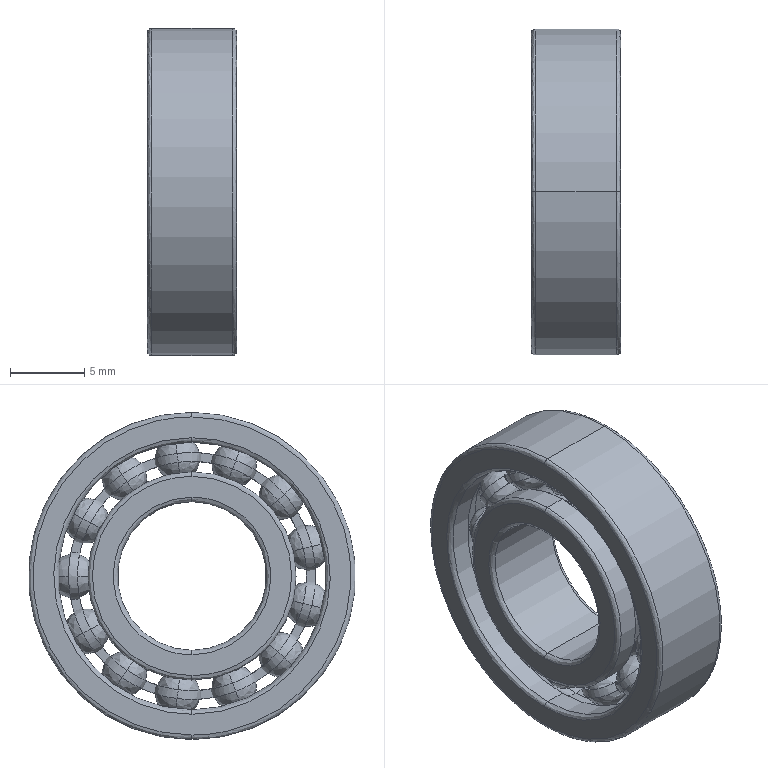Part | SolidWorks | features BaseBody 15 | 15 solids | 169 faces | box 6 x 22 x 22 mm | volume 1331 mm3 | spline 77 | cylinder 62 | plane 30 | commonest cylinder face diameters 15.4 x25 16.6 x25 14 x4 18 x4 10 x2 22 x2